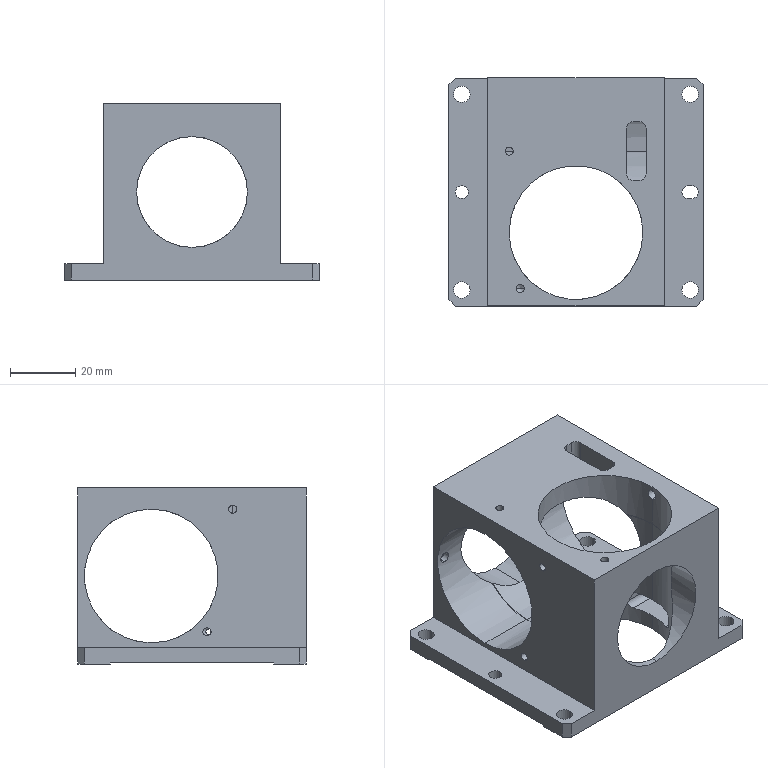NC program | NX | posted with a generic post | part box 78 x 70 x 54 mm
Whole program:
N10 G17 G21 G94 G90
(DRILLING_1 , TOOL : D6A45)
N12 T07 M6
N14 G54
N16 G17 G0 G90 X-35. Y30. B0. C0. S5000 M3
N18 G43 Z30. H7
N20 G94 G81 G98 Z-1.1 F250. R3.
N22 Y-30.
N24 X35.
N26 Y30.
N28 G80
N30 G0 X35. Y30. Z30.
N32 M5
(DRILLING_1_COPY , TOOL : 5.0ZT)
N34 T05 M6
N36 G54
N38 G17 G0 G90 X-35. Y30. B0. C0. S2000 M3
N40 G43 Z30. H5
N42 G94 G83 G98 Z-8.002 F250. Q2. R3.
N44 Y-30.
N46 X35.
N48 Y30.
N50 G80
N52 G0 X35. Y30. Z30.
N54 M5
(HOLE_MILLING_1 , TOOL : D3)
N56 T03 M6
N58 G54
N60 G17 G0 G90 X-35. Y0. B0. C0. S9500 M3
N62 G43 Z30. H3
N64 Z0.
N66 G94 G3 X-34.8 Y-0.2 R0.2 F1250.
N68 X-34.6 Y0. R0.2
N70 X-34.6 Y0. Z-0.15 I-0.4 J0.
N72 X-34.6 Y0. Z-0.3 I-0.4 J0.
N74 X-34.6 Y0. Z-0.45 I-0.4 J0.
N76 X-34.6 Y0. Z-0.6 I-0.4 J0.
N78 X-34.6 Y0. Z-0.75 I-0.4 J0.
N80 X-34.6 Y0. Z-0.9 I-0.4 J0.
N82 X-34.6 Y0. Z-1.05 I-0.4 J0.
N84 X-34.6 Y0. Z-1.2 I-0.4 J0.
N86 X-34.6 Y0. Z-1.35 I-0.4 J0.
N88 X-34.6 Y0. Z-1.5 I-0.4 J0.
N90 X-34.6 Y0. Z-1.65 I-0.4 J0.
N92 X-34.6 Y0. Z-1.8 I-0.4 J0.
N94 X-34.6 Y0. Z-1.95 I-0.4 J0.
N96 X-34.6 Y0. Z-2.1 I-0.4 J0.
N98 X-34.6 Y0. Z-2.25 I-0.4 J0.
N100 X-34.6 Y0. Z-2.4 I-0.4 J0.
N102 X-34.6 Y0. Z-2.55 I-0.4 J0.
N104 X-34.6 Y0. Z-2.7 I-0.4 J0.
N106 X-34.6 Y0. Z-2.85 I-0.4 J0.
N108 X-34.6 Y0. Z-3. I-0.4 J0.
N110 X-34.6 Y0. Z-3.15 I-0.4 J0.
N112 X-34.6 Y0. Z-3.3 I-0.4 J0.
N114 X-34.6 Y0. Z-3.45 I-0.4 J0.
N116 X-34.6 Y0. Z-3.6 I-0.4 J0.
N118 X-34.6 Y0. Z-3.75 I-0.4 J0.
N120 X-34.6 Y0. Z-3.9 I-0.4 J0.
N122 X-34.6 Y0. Z-4.05 I-0.4 J0.
N124 X-34.6 Y0. Z-4.2 I-0.4 J0.
N126 X-34.6 Y0. Z-4.35 I-0.4 J0.
N128 X-34.6 Y0. Z-4.5 I-0.4 J0.
N130 X-34.6 Y0. Z-4.65 I-0.4 J0.
N132 X-34.6 Y0. Z-4.8 I-0.4 J0.
N134 X-34.6 Y0. Z-4.95 I-0.4 J0.
N136 X-35.2 Y0.346 Z-5. R0.4
N138 X-35.346 Y-0.2 R0.4
N140 X-35.2 Y0.346 R-0.4
N142 X-35.273 Y0.073 R0.2
N144 X-35. Y0. R0.2
N146 G0 Z30.
(PLANAR_MILL_COPY_1_1_COPY , TOOL : D6A45)
N148 T07 M6
N150 G17 G43 G0 G90 X35.314 Y-30.247 Z30. B0. C0. S9500 H7 M3
N152 Z0.5
N154 G94 G1 Z-1. F1250.
N156 X36.1 Y-30.866
N158 G3 X36.6 Y-30. R1.
N160 X35. Y-28.4 R1.6
N162 X36.6 Y-30. R-1.6
N164 X36.1 Y-29.134 R1.
N166 G1 X35.314 Y-29.753
N168 Z0.5
N170 G0 Z30.
N172 X41.2 Y-24.84
N174 Z0.5
N176 G1 Z-1.
N178 X40.727 Y-24.874
N180 G3 X39.9 Y-25.436 R1.
N182 G1 Y-32.959
N184 G2 X39.607 Y-33.666 R1.
N186 G1 X37.666 Y-35.607
N188 G2 X36.959 Y-35.9 R1.
N190 G1 X-36.959
N192 G2 X-37.666 Y-35.607 R1.
N194 G1 X-39.607 Y-33.666
N196 G2 X-39.9 Y-32.959 R1.
N198 G1 Y-25.436
N200 G3 X-40.727 Y-24.874 R1.
N202 G1 X-41.2 Y-24.84
N204 Z0.5
N206 G0 Z30.
N208 Y24.84
N210 Z0.5
N212 G1 Z-1.
N214 X-40.727 Y24.874
N216 G3 X-39.9 Y25.436 R1.
N218 G1 Y32.959
N220 G2 X-39.607 Y33.666 R1.
N222 G1 X-37.666 Y35.607
N224 G2 X-36.959 Y35.9 R1.
N226 G1 X36.959
N228 G2 X37.666 Y35.607 R1.
N230 G1 X39.607 Y33.666
N232 G2 X39.9 Y32.959 R1.
N234 G1 Y25.436
N236 G3 X40.727 Y24.874 R1.
N238 G1 X41.2 Y24.84
N240 Z0.5
N242 G0 Z30.
N244 X35.314 Y29.753
N246 Z0.5
N248 G1 Z-1.
N250 X36.1 Y29.134
N252 G3 X36.6 Y30. R1.
N254 X35. Y31.6 R1.6
N256 X36.6 Y30. R-1.6
N258 X36.1 Y30.866 R1.
N260 G1 X35.314 Y30.247
N262 Z0.5
N264 G0 Z30.
N266 X14.856 Y23.525
N268 Z0.5
N270 G1 Z-1.
N272 X15.211 Y23.843
N274 G3 X15.521 Y24.794 R1.
N276 X-15.521 Y24.794 R19.8
N278 X-15.211 Y23.843 R1.
N280 G1 X-14.856 Y23.525
N282 Z0.5
N284 G0 Z30.
N286 X-35.314 Y30.247
N288 Z0.5
N290 G1 Z-1.
N292 X-36.1 Y30.866
N294 G3 X-36.6 Y30. R1.
N296 X-35. Y28.4 R1.6
N298 X-36.6 Y30. R-1.6
N300 X-36.1 Y29.134 R1.
N302 G1 X-35.314 Y29.753
N304 Z0.5
N306 G0 Z30.
N308 Y-29.753
N310 Z0.5
N312 G1 Z-1.
N314 X-36.1 Y-29.134
N316 G3 X-36.6 Y-30. R1.
N318 X-35. Y-31.6 R1.6
N320 X-36.6 Y-30. R-1.6
N322 X-36.1 Y-30.866 R1.
N324 G1 X-35.314 Y-30.247
N326 Z0.5
N328 G0 Z30.
(PLANAR_MILL_COPY_1_1_COPY_COPY , TOOL : D6A45)
N330 X-35.325 Y-1.063
N332 Z0.
N334 G1 X-35.259 Y-1.1 Z-0.02
N336 X-35. Z-0.09
N338 X-34.741 Z-0.159
N340 X-34.201 Y-0.799 Z-0.325
N342 X-33.9 Y-0.259 Z-0.491
N344 Y0.259 Z-0.629
N346 X-34.201 Y0.799 Z-0.795
N348 X-34.741 Y1.1 Z-0.961
N350 X-35.259 Z-1.099
N352 X-35.799 Y0.799 Z-1.265
N354 X-36.1 Y0.259 Z-1.431
N356 Y0. Z-1.5
N358 G3 X-35. Y-1.1 R1.1
N360 X-36.1 Y0. R-1.1
N362 X-35.6 Y-0.866 R1.
N364 G1 Z0.
N366 G0 Z30.
N368 X-15.592 Y21.931
N370 Z0.
N372 G1 Z-1.5
N374 X-15.921 Y22.5
N376 G3 X-16.787 Y23. R1.
N378 X16.787 Y23. R-19.8
N380 X15.921 Y22.5 R1.
N382 G1 X15.592 Y21.931
N384 Z0.
N386 G0 Z30.
N388 X41.369 Y22.849
N390 Z0.
N392 G1 Z-1.5
N394 X40.898 Y23.157
N396 G3 X39.9 Y23.214 R1.
N398 G1 Y-23.214
N400 G3 X40.898 Y-23.157 R1.
N402 G1 X41.369 Y-22.849
N404 Z0.
N406 G0 Z30.
N408 X-41.369
N410 Z0.
N412 G1 Z-1.5
N414 X-40.898 Y-23.157
N416 G3 X-39.9 Y-23.214 R1.
N418 G1 Y23.214
N420 G3 X-40.898 Y23.157 R1.
N422 G1 X-41.369 Y22.849
N424 Z0.
N426 G0 Z30.
N428 X36.048 Y0.939
N430 Z0.
N432 G1 X35.759 Y1.1 Z-0.089
N434 X34.241 Z-0.495
N436 X33.701 Y0.799 Z-0.661
N438 X33.4 Y0.259 Z-0.827
N440 Y-0.259 Z-0.965
N442 X33.701 Y-0.799 Z-1.131
N444 X34.241 Y-1.1 Z-1.297
N446 X35. Z-1.5
N448 X35.5
N450 G3 X36.6 Y0. R1.1
N452 X35.5 Y1.1 R1.1
N454 G1 X34.5
N456 G3 X33.4 Y0. R1.1
N458 X34.5 Y-1.1 R1.1
N460 G1 X35.
N462 G3 X35.866 Y-0.6 R1.
N464 G1 Z0.
N466 G0 Z30.
N468 M5
(TOOLCOMP_1 , TOOL : D3)
N470 T03 M6
N472 G54
N474 G17 G0 G90 X-35. Y0. B0. C0. S9500 M3
N476 G43 Z30. H3
N478 Z0.
N480 G41 G94 G1 X-34.973 Y-0.096 F1250. D3
N482 G3 X-34.55 Y0. R0.222
N484 X-34.55 Y0. Z-2. I-0.45 J0.
N486 X-34.55 Y0. Z-4. I-0.45 J0.
N488 X-35.45 Y0. Z-5. I-0.45 J0.
N490 X-35. Y-0.45 R0.45
N492 X-35.45 Y0. R-0.45
N494 X-35.027 Y-0.096 R0.222
N496 G40
N498 G1 X-35. Y0.
N500 G0 Z30.
(TOOLCOMP1 , TOOL : D3)
N502 X35.098 Y0.433
N504 Z-0.5
N506 G1 Z-5. F1200.
N508 G41 X35. Y0.45
N510 X34.5
N512 G3 X34.05 Y0. R0.45
N514 X34.5 Y-0.45 R0.45
N516 G1 X35.5
N518 G3 X35.95 Y0. R0.45
N520 X35.5 Y0.45 R0.45
N522 G1 X35.
N524 G3 X34.74 Y0.3 R0.3
N526 G40
N528 G1 X34.706 Y0.206
N530 G0 Z30.
N532 M5
N534 M2